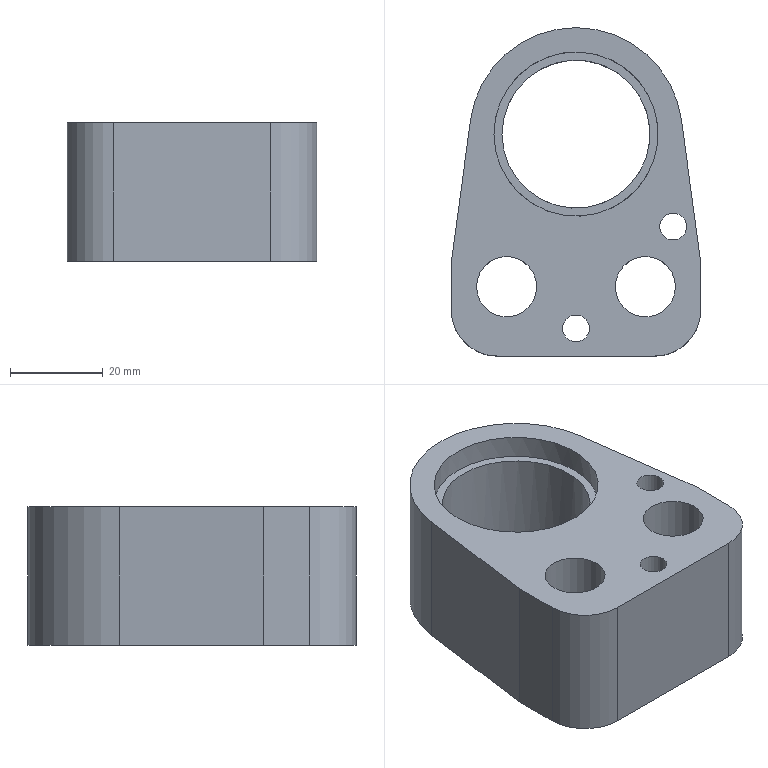Part | NX | features solid 2 | 1 solid | 25 faces | box 54 x 71 x 30 mm | volume 58450 mm3 | cylinder 13 | plane 12 | commonest cylinder face diameters 5.8 x2 8 x2 13 x2 19 x2 20 x2 32 x1
STEP:
#1=CARTESIAN_POINT('',(83.431,151.38,95.));
#2=VERTEX_POINT('',#1);
#3=CARTESIAN_POINT('',(79.223,182.47,95.));
#4=VERTEX_POINT('',#3);
#5=CARTESIAN_POINT('',(80.748,171.199,95.));
#6=DIRECTION('',(-0.1341,0.991,0.));
#7=VECTOR('',#6,1000.);
#8=LINE('',#5,#7);
#9=EDGE_CURVE('',#2,#4,#8,.T.);
#10=ORIENTED_EDGE('',*,*,#9,.T.);
#11=CARTESIAN_POINT('',(33.64,182.47,95.));
#12=VERTEX_POINT('',#11);
#13=CARTESIAN_POINT('',(56.431,179.38,95.));
#14=DIRECTION('',(0.,0.,-1.));
#15=DIRECTION('',(-1.,0.,0.));
#16=AXIS2_PLACEMENT_3D('',#13,#14,#15);
#17=CIRCLE('',#16,23.);
#18=EDGE_CURVE('',#12,#4,#17,.T.);
#19=ORIENTED_EDGE('',*,*,#18,.F.);
#20=CARTESIAN_POINT('',(29.431,151.38,95.));
#21=VERTEX_POINT('',#20);
#22=CARTESIAN_POINT('',(32.114,171.199,95.));
#23=DIRECTION('',(-0.1341,-0.991,0.));
#24=VECTOR('',#23,1000.);
#25=LINE('',#22,#24);
#26=EDGE_CURVE('',#12,#21,#25,.T.);
#27=ORIENTED_EDGE('',*,*,#26,.T.);
#28=CARTESIAN_POINT('',(29.431,141.38,95.));
#29=VERTEX_POINT('',#28);
#30=CARTESIAN_POINT('',(29.431,166.925,95.));
#31=DIRECTION('',(0.,1.,0.));
#32=VECTOR('',#31,1000.);
#33=LINE('',#30,#32);
#34=EDGE_CURVE('',#29,#21,#33,.T.);
#35=ORIENTED_EDGE('',*,*,#34,.F.);
#36=CARTESIAN_POINT('',(39.431,131.38,95.));
#37=VERTEX_POINT('',#36);
#38=CARTESIAN_POINT('',(39.431,141.38,95.));
#39=DIRECTION('',(0.,0.,1.));
#40=DIRECTION('',(1.,0.,0.));
#41=AXIS2_PLACEMENT_3D('',#38,#39,#40);
#42=CIRCLE('',#41,10.);
#43=EDGE_CURVE('',#29,#37,#42,.T.);
#44=ORIENTED_EDGE('',*,*,#43,.T.);
#45=CARTESIAN_POINT('',(73.431,131.38,95.));
#46=VERTEX_POINT('',#45);
#47=CARTESIAN_POINT('',(56.431,131.38,95.));
#48=DIRECTION('',(-1.,0.,0.));
#49=VECTOR('',#48,1000.);
#50=LINE('',#47,#49);
#51=EDGE_CURVE('',#46,#37,#50,.T.);
#52=ORIENTED_EDGE('',*,*,#51,.F.);
#53=CARTESIAN_POINT('',(83.431,141.38,95.));
#54=VERTEX_POINT('',#53);
#55=CARTESIAN_POINT('',(73.431,141.38,95.));
#56=DIRECTION('',(0.,0.,1.));
#57=DIRECTION('',(1.,0.,0.));
#58=AXIS2_PLACEMENT_3D('',#55,#56,#57);
#59=CIRCLE('',#58,10.);
#60=EDGE_CURVE('',#46,#54,#59,.T.);
#61=ORIENTED_EDGE('',*,*,#60,.T.);
#62=CARTESIAN_POINT('',(83.431,166.925,95.));
#63=DIRECTION('',(0.,-1.,0.));
#64=VECTOR('',#63,1000.);
#65=LINE('',#62,#64);
#66=EDGE_CURVE('',#2,#54,#65,.T.);
#67=ORIENTED_EDGE('',*,*,#66,.F.);
#68=EDGE_LOOP('',(#10,#19,#27,#35,#44,#52,#61,#67));
#69=FACE_BOUND('',#68,.T.);
#70=CARTESIAN_POINT('',(53.531,137.38,95.));
#71=VERTEX_POINT('',#70);
#72=CARTESIAN_POINT('',(56.431,137.38,95.));
#73=DIRECTION('',(0.,0.,-1.));
#74=DIRECTION('',(-1.,0.,0.));
#75=AXIS2_PLACEMENT_3D('',#72,#73,#74);
#76=CIRCLE('',#75,2.9);
#77=EDGE_CURVE('',#71,#71,#76,.T.);
#78=ORIENTED_EDGE('',*,*,#77,.T.);
#79=EDGE_LOOP('',(#78));
#80=FACE_BOUND('',#79,.T.);
#81=CARTESIAN_POINT('',(74.531,159.38,95.));
#82=VERTEX_POINT('',#81);
#83=CARTESIAN_POINT('',(77.431,159.38,95.));
#84=DIRECTION('',(0.,0.,-1.));
#85=DIRECTION('',(-1.,0.,0.));
#86=AXIS2_PLACEMENT_3D('',#83,#84,#85);
#87=CIRCLE('',#86,2.9);
#88=EDGE_CURVE('',#82,#82,#87,.T.);
#89=ORIENTED_EDGE('',*,*,#88,.T.);
#90=EDGE_LOOP('',(#89));
#91=FACE_BOUND('',#90,.T.);
#92=CARTESIAN_POINT('',(64.931,146.38,95.));
#93=VERTEX_POINT('',#92);
#94=CARTESIAN_POINT('',(71.431,146.38,95.));
#95=DIRECTION('',(0.,0.,-1.));
#96=DIRECTION('',(-1.,0.,0.));
#97=AXIS2_PLACEMENT_3D('',#94,#95,#96);
#98=CIRCLE('',#97,6.5);
#99=EDGE_CURVE('',#93,#93,#98,.T.);
#100=ORIENTED_EDGE('',*,*,#99,.T.);
#101=EDGE_LOOP('',(#100));
#102=FACE_BOUND('',#101,.T.);
#103=CARTESIAN_POINT('',(34.931,146.38,95.));
#104=VERTEX_POINT('',#103);
#105=CARTESIAN_POINT('',(41.431,146.38,95.));
#106=DIRECTION('',(0.,0.,-1.));
#107=DIRECTION('',(-1.,0.,0.));
#108=AXIS2_PLACEMENT_3D('',#105,#106,#107);
#109=CIRCLE('',#108,6.5);
#110=EDGE_CURVE('',#104,#104,#109,.T.);
#111=ORIENTED_EDGE('',*,*,#110,.T.);
#112=EDGE_LOOP('',(#111));
#113=FACE_BOUND('',#112,.T.);
#114=CARTESIAN_POINT('',(38.681,179.38,95.));
#115=VERTEX_POINT('',#114);
#116=CARTESIAN_POINT('',(56.431,179.38,95.));
#117=DIRECTION('',(0.,0.,-1.));
#118=DIRECTION('',(-1.,0.,0.));
#119=AXIS2_PLACEMENT_3D('',#116,#117,#118);
#120=CIRCLE('',#119,17.75);
#121=EDGE_CURVE('',#115,#115,#120,.T.);
#122=ORIENTED_EDGE('',*,*,#121,.T.);
#123=EDGE_LOOP('',(#122));
#124=FACE_BOUND('',#123,.T.);
#125=CARTESIAN_POINT('',(56.431,166.925,95.));
#126=DIRECTION('',(0.,0.,1.));
#127=DIRECTION('',(1.,0.,0.));
#128=AXIS2_PLACEMENT_3D('',#125,#126,#127);
#129=PLANE('',#128);
#130=ADVANCED_FACE('',(#69,#80,#91,#102,#113,#124),#129,.T.);
#131=CARTESIAN_POINT('',(29.431,151.38,65.));
#132=VERTEX_POINT('',#131);
#133=CARTESIAN_POINT('',(29.431,151.38,65.));
#134=DIRECTION('',(0.,0.,1.));
#135=VECTOR('',#134,1000.);
#136=LINE('',#133,#135);
#137=EDGE_CURVE('',#132,#21,#136,.T.);
#138=ORIENTED_EDGE('',*,*,#137,.F.);
#139=CARTESIAN_POINT('',(29.431,141.38,65.));
#140=VERTEX_POINT('',#139);
#141=CARTESIAN_POINT('',(29.431,166.925,65.));
#142=DIRECTION('',(0.,-1.,0.));
#143=VECTOR('',#142,1000.);
#144=LINE('',#141,#143);
#145=EDGE_CURVE('',#132,#140,#144,.T.);
#146=ORIENTED_EDGE('',*,*,#145,.T.);
#147=CARTESIAN_POINT('',(29.431,141.38,65.));
#148=DIRECTION('',(0.,0.,1.));
#149=VECTOR('',#148,1000.);
#150=LINE('',#147,#149);
#151=EDGE_CURVE('',#140,#29,#150,.T.);
#152=ORIENTED_EDGE('',*,*,#151,.T.);
#153=ORIENTED_EDGE('',*,*,#34,.T.);
#154=EDGE_LOOP('',(#138,#146,#152,#153));
#155=FACE_BOUND('',#154,.T.);
#156=CARTESIAN_POINT('',(29.431,166.925,65.));
#157=DIRECTION('',(-1.,0.,0.));
#158=DIRECTION('',(0.,0.,1.));
#159=AXIS2_PLACEMENT_3D('',#156,#157,#158);
#160=PLANE('',#159);
#161=ADVANCED_FACE('',(#155),#160,.T.);
#162=CARTESIAN_POINT('',(79.223,182.47,65.));
#163=VERTEX_POINT('',#162);
#164=CARTESIAN_POINT('',(83.431,151.38,65.));
#165=VERTEX_POINT('',#164);
#166=CARTESIAN_POINT('',(80.748,171.199,65.));
#167=DIRECTION('',(0.1341,-0.991,0.));
#168=VECTOR('',#167,1000.);
#169=LINE('',#166,#168);
#170=EDGE_CURVE('',#163,#165,#169,.T.);
#171=ORIENTED_EDGE('',*,*,#170,.T.);
#172=CARTESIAN_POINT('',(83.431,141.38,65.));
#173=VERTEX_POINT('',#172);
#174=CARTESIAN_POINT('',(83.431,166.925,65.));
#175=DIRECTION('',(0.,1.,0.));
#176=VECTOR('',#175,1000.);
#177=LINE('',#174,#176);
#178=EDGE_CURVE('',#173,#165,#177,.T.);
#179=ORIENTED_EDGE('',*,*,#178,.F.);
#180=CARTESIAN_POINT('',(73.431,131.38,65.));
#181=VERTEX_POINT('',#180);
#182=CARTESIAN_POINT('',(73.431,141.38,65.));
#183=DIRECTION('',(0.,0.,-1.));
#184=DIRECTION('',(-1.,0.,0.));
#185=AXIS2_PLACEMENT_3D('',#182,#183,#184);
#186=CIRCLE('',#185,10.);
#187=EDGE_CURVE('',#173,#181,#186,.T.);
#188=ORIENTED_EDGE('',*,*,#187,.T.);
#189=CARTESIAN_POINT('',(39.431,131.38,65.));
#190=VERTEX_POINT('',#189);
#191=CARTESIAN_POINT('',(56.431,131.38,65.));
#192=DIRECTION('',(1.,0.,0.));
#193=VECTOR('',#192,1000.);
#194=LINE('',#191,#193);
#195=EDGE_CURVE('',#190,#181,#194,.T.);
#196=ORIENTED_EDGE('',*,*,#195,.F.);
#197=CARTESIAN_POINT('',(39.431,141.38,65.));
#198=DIRECTION('',(0.,0.,-1.));
#199=DIRECTION('',(-1.,0.,0.));
#200=AXIS2_PLACEMENT_3D('',#197,#198,#199);
#201=CIRCLE('',#200,10.);
#202=EDGE_CURVE('',#190,#140,#201,.T.);
#203=ORIENTED_EDGE('',*,*,#202,.T.);
#204=ORIENTED_EDGE('',*,*,#145,.F.);
#205=CARTESIAN_POINT('',(33.64,182.47,65.));
#206=VERTEX_POINT('',#205);
#207=CARTESIAN_POINT('',(32.114,171.199,65.));
#208=DIRECTION('',(0.1341,0.991,0.));
#209=VECTOR('',#208,1000.);
#210=LINE('',#207,#209);
#211=EDGE_CURVE('',#132,#206,#210,.T.);
#212=ORIENTED_EDGE('',*,*,#211,.T.);
#213=CARTESIAN_POINT('',(56.431,179.38,65.));
#214=DIRECTION('',(0.,0.,1.));
#215=DIRECTION('',(1.,0.,0.));
#216=AXIS2_PLACEMENT_3D('',#213,#214,#215);
#217=CIRCLE('',#216,23.);
#218=EDGE_CURVE('',#163,#206,#217,.T.);
#219=ORIENTED_EDGE('',*,*,#218,.F.);
#220=EDGE_LOOP('',(#171,#179,#188,#196,#203,#204,#212,#219));
#221=FACE_BOUND('',#220,.T.);
#222=CARTESIAN_POINT('',(60.431,137.38,65.));
#223=VERTEX_POINT('',#222);
#224=CARTESIAN_POINT('',(56.431,137.38,65.));
#225=DIRECTION('',(0.,0.,1.));
#226=DIRECTION('',(1.,0.,0.));
#227=AXIS2_PLACEMENT_3D('',#224,#225,#226);
#228=CIRCLE('',#227,4.);
#229=EDGE_CURVE('',#223,#223,#228,.T.);
#230=ORIENTED_EDGE('',*,*,#229,.T.);
#231=EDGE_LOOP('',(#230));
#232=FACE_BOUND('',#231,.T.);
#233=CARTESIAN_POINT('',(81.431,159.38,65.));
#234=VERTEX_POINT('',#233);
#235=CARTESIAN_POINT('',(77.431,159.38,65.));
#236=DIRECTION('',(0.,0.,1.));
#237=DIRECTION('',(1.,0.,0.));
#238=AXIS2_PLACEMENT_3D('',#235,#236,#237);
#239=CIRCLE('',#238,4.);
#240=EDGE_CURVE('',#234,#234,#239,.T.);
#241=ORIENTED_EDGE('',*,*,#240,.T.);
#242=EDGE_LOOP('',(#241));
#243=FACE_BOUND('',#242,.T.);
#244=CARTESIAN_POINT('',(80.931,146.38,65.));
#245=VERTEX_POINT('',#244);
#246=CARTESIAN_POINT('',(71.431,146.38,65.));
#247=DIRECTION('',(0.,0.,1.));
#248=DIRECTION('',(1.,0.,0.));
#249=AXIS2_PLACEMENT_3D('',#246,#247,#248);
#250=CIRCLE('',#249,9.5);
#251=EDGE_CURVE('',#245,#245,#250,.T.);
#252=ORIENTED_EDGE('',*,*,#251,.T.);
#253=EDGE_LOOP('',(#252));
#254=FACE_BOUND('',#253,.T.);
#255=CARTESIAN_POINT('',(50.931,146.38,65.));
#256=VERTEX_POINT('',#255);
#257=CARTESIAN_POINT('',(41.431,146.38,65.));
#258=DIRECTION('',(0.,0.,1.));
#259=DIRECTION('',(1.,0.,0.));
#260=AXIS2_PLACEMENT_3D('',#257,#258,#259);
#261=CIRCLE('',#260,9.5);
#262=EDGE_CURVE('',#256,#256,#261,.T.);
#263=ORIENTED_EDGE('',*,*,#262,.T.);
#264=EDGE_LOOP('',(#263));
#265=FACE_BOUND('',#264,.T.);
#266=CARTESIAN_POINT('',(72.431,179.38,65.));
#267=VERTEX_POINT('',#266);
#268=CARTESIAN_POINT('',(56.431,179.38,65.));
#269=DIRECTION('',(0.,0.,1.));
#270=DIRECTION('',(1.,0.,0.));
#271=AXIS2_PLACEMENT_3D('',#268,#269,#270);
#272=CIRCLE('',#271,16.);
#273=EDGE_CURVE('',#267,#267,#272,.T.);
#274=ORIENTED_EDGE('',*,*,#273,.T.);
#275=EDGE_LOOP('',(#274));
#276=FACE_BOUND('',#275,.T.);
#277=CARTESIAN_POINT('',(56.431,166.925,65.));
#278=DIRECTION('',(0.,0.,-1.));
#279=DIRECTION('',(-1.,0.,0.));
#280=AXIS2_PLACEMENT_3D('',#277,#278,#279);
#281=PLANE('',#280);
#282=ADVANCED_FACE('',(#221,#232,#243,#254,#265,#276),#281,.T.);
#283=CARTESIAN_POINT('',(83.431,151.38,65.));
#284=DIRECTION('',(0.,0.,1.));
#285=VECTOR('',#284,1000.);
#286=LINE('',#283,#285);
#287=EDGE_CURVE('',#165,#2,#286,.T.);
#288=ORIENTED_EDGE('',*,*,#287,.T.);
#289=ORIENTED_EDGE('',*,*,#66,.T.);
#290=CARTESIAN_POINT('',(83.431,141.38,65.));
#291=DIRECTION('',(0.,0.,1.));
#292=VECTOR('',#291,1000.);
#293=LINE('',#290,#292);
#294=EDGE_CURVE('',#54,#173,#293,.F.);
#295=ORIENTED_EDGE('',*,*,#294,.T.);
#296=ORIENTED_EDGE('',*,*,#178,.T.);
#297=EDGE_LOOP('',(#288,#289,#295,#296));
#298=FACE_BOUND('',#297,.T.);
#299=CARTESIAN_POINT('',(83.431,166.925,65.));
#300=DIRECTION('',(1.,0.,0.));
#301=DIRECTION('',(0.,0.,-1.));
#302=AXIS2_PLACEMENT_3D('',#299,#300,#301);
#303=PLANE('',#302);
#304=ADVANCED_FACE('',(#298),#303,.T.);
#305=ORIENTED_EDGE('',*,*,#18,.T.);
#306=CARTESIAN_POINT('',(79.223,182.47,95.));
#307=DIRECTION('',(0.,0.,-1.));
#308=VECTOR('',#307,1000.);
#309=LINE('',#306,#308);
#310=EDGE_CURVE('',#4,#163,#309,.T.);
#311=ORIENTED_EDGE('',*,*,#310,.T.);
#312=ORIENTED_EDGE('',*,*,#218,.T.);
#313=CARTESIAN_POINT('',(33.64,182.47,95.));
#314=DIRECTION('',(0.,0.,-1.));
#315=VECTOR('',#314,1000.);
#316=LINE('',#313,#315);
#317=EDGE_CURVE('',#206,#12,#316,.F.);
#318=ORIENTED_EDGE('',*,*,#317,.T.);
#319=EDGE_LOOP('',(#305,#311,#312,#318));
#320=FACE_BOUND('',#319,.T.);
#321=CARTESIAN_POINT('',(56.431,179.38,95.));
#322=DIRECTION('',(0.,0.,-1.));
#323=DIRECTION('',(-1.,0.,0.));
#324=AXIS2_PLACEMENT_3D('',#321,#322,#323);
#325=CYLINDRICAL_SURFACE('',#324,23.);
#326=ADVANCED_FACE('',(#320),#325,.T.);
#327=ORIENTED_EDGE('',*,*,#195,.T.);
#328=CARTESIAN_POINT('',(73.431,131.38,65.));
#329=DIRECTION('',(0.,0.,1.));
#330=VECTOR('',#329,1000.);
#331=LINE('',#328,#330);
#332=EDGE_CURVE('',#181,#46,#331,.T.);
#333=ORIENTED_EDGE('',*,*,#332,.T.);
#334=ORIENTED_EDGE('',*,*,#51,.T.);
#335=CARTESIAN_POINT('',(39.431,131.38,65.));
#336=DIRECTION('',(0.,0.,1.));
#337=VECTOR('',#336,1000.);
#338=LINE('',#335,#337);
#339=EDGE_CURVE('',#37,#190,#338,.F.);
#340=ORIENTED_EDGE('',*,*,#339,.T.);
#341=EDGE_LOOP('',(#327,#333,#334,#340));
#342=FACE_BOUND('',#341,.T.);
#343=CARTESIAN_POINT('',(56.431,131.38,65.));
#344=DIRECTION('',(0.,-1.,0.));
#345=DIRECTION('',(0.,0.,-1.));
#346=AXIS2_PLACEMENT_3D('',#343,#344,#345);
#347=PLANE('',#346);
#348=ADVANCED_FACE('',(#342),#347,.T.);
#349=CARTESIAN_POINT('',(40.431,179.38,90.));
#350=VERTEX_POINT('',#349);
#351=CARTESIAN_POINT('',(56.431,179.38,90.));
#352=DIRECTION('',(0.,0.,-1.));
#353=DIRECTION('',(-1.,0.,0.));
#354=AXIS2_PLACEMENT_3D('',#351,#352,#353);
#355=CIRCLE('',#354,16.);
#356=EDGE_CURVE('',#350,#350,#355,.T.);
#357=ORIENTED_EDGE('',*,*,#356,.T.);
#358=EDGE_LOOP('',(#357));
#359=FACE_BOUND('',#358,.T.);
#360=CARTESIAN_POINT('',(74.181,179.38,90.));
#361=VERTEX_POINT('',#360);
#362=CARTESIAN_POINT('',(56.431,179.38,90.));
#363=DIRECTION('',(0.,0.,1.));
#364=DIRECTION('',(1.,0.,0.));
#365=AXIS2_PLACEMENT_3D('',#362,#363,#364);
#366=CIRCLE('',#365,17.75);
#367=EDGE_CURVE('',#361,#361,#366,.T.);
#368=ORIENTED_EDGE('',*,*,#367,.T.);
#369=EDGE_LOOP('',(#368));
#370=FACE_BOUND('',#369,.T.);
#371=CARTESIAN_POINT('',(56.431,179.38,90.));
#372=DIRECTION('',(0.,0.,-1.));
#373=DIRECTION('',(-1.,0.,0.));
#374=AXIS2_PLACEMENT_3D('',#371,#372,#373);
#375=PLANE('',#374);
#376=ADVANCED_FACE('',(#359,#370),#375,.F.);
#377=ORIENTED_EDGE('',*,*,#367,.F.);
#378=EDGE_LOOP('',(#377));
#379=FACE_BOUND('',#378,.T.);
#380=ORIENTED_EDGE('',*,*,#121,.F.);
#381=EDGE_LOOP('',(#380));
#382=FACE_BOUND('',#381,.T.);
#383=CARTESIAN_POINT('',(56.431,179.38,95.));
#384=DIRECTION('',(0.,0.,-1.));
#385=DIRECTION('',(-1.,0.,0.));
#386=AXIS2_PLACEMENT_3D('',#383,#384,#385);
#387=CYLINDRICAL_SURFACE('',#386,17.75);
#388=ADVANCED_FACE('',(#379,#382),#387,.F.);
#389=ORIENTED_EDGE('',*,*,#273,.F.);
#390=EDGE_LOOP('',(#389));
#391=FACE_BOUND('',#390,.T.);
#392=ORIENTED_EDGE('',*,*,#356,.F.);
#393=EDGE_LOOP('',(#392));
#394=FACE_BOUND('',#393,.T.);
#395=CARTESIAN_POINT('',(56.431,179.38,90.));
#396=DIRECTION('',(0.,0.,-1.));
#397=DIRECTION('',(-1.,0.,0.));
#398=AXIS2_PLACEMENT_3D('',#395,#396,#397);
#399=CYLINDRICAL_SURFACE('',#398,16.);
#400=ADVANCED_FACE('',(#391,#394),#399,.F.);
#401=CARTESIAN_POINT('',(47.931,146.38,79.));
#402=VERTEX_POINT('',#401);
#403=CARTESIAN_POINT('',(41.431,146.38,79.));
#404=DIRECTION('',(0.,0.,1.));
#405=DIRECTION('',(1.,0.,0.));
#406=AXIS2_PLACEMENT_3D('',#403,#404,#405);
#407=CIRCLE('',#406,6.5);
#408=EDGE_CURVE('',#402,#402,#407,.F.);
#409=ORIENTED_EDGE('',*,*,#408,.T.);
#410=EDGE_LOOP('',(#409));
#411=FACE_BOUND('',#410,.T.);
#412=ORIENTED_EDGE('',*,*,#110,.F.);
#413=EDGE_LOOP('',(#412));
#414=FACE_BOUND('',#413,.T.);
#415=CARTESIAN_POINT('',(41.431,146.38,95.));
#416=DIRECTION('',(0.,0.,-1.));
#417=DIRECTION('',(-1.,0.,0.));
#418=AXIS2_PLACEMENT_3D('',#415,#416,#417);
#419=CYLINDRICAL_SURFACE('',#418,6.5);
#420=ADVANCED_FACE('',(#411,#414),#419,.F.);
#421=CARTESIAN_POINT('',(31.931,146.38,79.));
#422=VERTEX_POINT('',#421);
#423=CARTESIAN_POINT('',(41.431,146.38,79.));
#424=DIRECTION('',(0.,0.,-1.));
#425=DIRECTION('',(-1.,0.,0.));
#426=AXIS2_PLACEMENT_3D('',#423,#424,#425);
#427=CIRCLE('',#426,9.5);
#428=EDGE_CURVE('',#422,#422,#427,.T.);
#429=ORIENTED_EDGE('',*,*,#428,.T.);
#430=EDGE_LOOP('',(#429));
#431=FACE_BOUND('',#430,.T.);
#432=ORIENTED_EDGE('',*,*,#408,.F.);
#433=EDGE_LOOP('',(#432));
#434=FACE_BOUND('',#433,.T.);
#435=CARTESIAN_POINT('',(41.431,146.38,79.));
#436=DIRECTION('',(0.,0.,1.));
#437=DIRECTION('',(1.,0.,0.));
#438=AXIS2_PLACEMENT_3D('',#435,#436,#437);
#439=PLANE('',#438);
#440=ADVANCED_FACE('',(#431,#434),#439,.F.);
#441=ORIENTED_EDGE('',*,*,#262,.F.);
#442=EDGE_LOOP('',(#441));
#443=FACE_BOUND('',#442,.T.);
#444=ORIENTED_EDGE('',*,*,#428,.F.);
#445=EDGE_LOOP('',(#444));
#446=FACE_BOUND('',#445,.T.);
#447=CARTESIAN_POINT('',(41.431,146.38,79.));
#448=DIRECTION('',(0.,0.,-1.));
#449=DIRECTION('',(-1.,0.,0.));
#450=AXIS2_PLACEMENT_3D('',#447,#448,#449);
#451=CYLINDRICAL_SURFACE('',#450,9.5);
#452=ADVANCED_FACE('',(#443,#446),#451,.F.);
#453=CARTESIAN_POINT('',(77.931,146.38,79.));
#454=VERTEX_POINT('',#453);
#455=CARTESIAN_POINT('',(71.431,146.38,79.));
#456=DIRECTION('',(0.,0.,1.));
#457=DIRECTION('',(1.,0.,0.));
#458=AXIS2_PLACEMENT_3D('',#455,#456,#457);
#459=CIRCLE('',#458,6.5);
#460=EDGE_CURVE('',#454,#454,#459,.F.);
#461=ORIENTED_EDGE('',*,*,#460,.T.);
#462=EDGE_LOOP('',(#461));
#463=FACE_BOUND('',#462,.T.);
#464=ORIENTED_EDGE('',*,*,#99,.F.);
#465=EDGE_LOOP('',(#464));
#466=FACE_BOUND('',#465,.T.);
#467=CARTESIAN_POINT('',(71.431,146.38,95.));
#468=DIRECTION('',(0.,0.,-1.));
#469=DIRECTION('',(-1.,0.,0.));
#470=AXIS2_PLACEMENT_3D('',#467,#468,#469);
#471=CYLINDRICAL_SURFACE('',#470,6.5);
#472=ADVANCED_FACE('',(#463,#466),#471,.F.);
#473=CARTESIAN_POINT('',(61.931,146.38,79.));
#474=VERTEX_POINT('',#473);
#475=CARTESIAN_POINT('',(71.431,146.38,79.));
#476=DIRECTION('',(0.,0.,-1.));
#477=DIRECTION('',(-1.,0.,0.));
#478=AXIS2_PLACEMENT_3D('',#475,#476,#477);
#479=CIRCLE('',#478,9.5);
#480=EDGE_CURVE('',#474,#474,#479,.T.);
#481=ORIENTED_EDGE('',*,*,#480,.T.);
#482=EDGE_LOOP('',(#481));
#483=FACE_BOUND('',#482,.T.);
#484=ORIENTED_EDGE('',*,*,#460,.F.);
#485=EDGE_LOOP('',(#484));
#486=FACE_BOUND('',#485,.T.);
#487=CARTESIAN_POINT('',(71.431,146.38,79.));
#488=DIRECTION('',(0.,0.,1.));
#489=DIRECTION('',(1.,0.,0.));
#490=AXIS2_PLACEMENT_3D('',#487,#488,#489);
#491=PLANE('',#490);
#492=ADVANCED_FACE('',(#483,#486),#491,.F.);
#493=ORIENTED_EDGE('',*,*,#251,.F.);
#494=EDGE_LOOP('',(#493));
#495=FACE_BOUND('',#494,.T.);
#496=ORIENTED_EDGE('',*,*,#480,.F.);
#497=EDGE_LOOP('',(#496));
#498=FACE_BOUND('',#497,.T.);
#499=CARTESIAN_POINT('',(71.431,146.38,79.));
#500=DIRECTION('',(0.,0.,-1.));
#501=DIRECTION('',(-1.,0.,0.));
#502=AXIS2_PLACEMENT_3D('',#499,#500,#501);
#503=CYLINDRICAL_SURFACE('',#502,9.5);
#504=ADVANCED_FACE('',(#495,#498),#503,.F.);
#505=CARTESIAN_POINT('',(80.331,159.38,85.));
#506=VERTEX_POINT('',#505);
#507=CARTESIAN_POINT('',(77.431,159.38,85.));
#508=DIRECTION('',(0.,0.,1.));
#509=DIRECTION('',(1.,0.,0.));
#510=AXIS2_PLACEMENT_3D('',#507,#508,#509);
#511=CIRCLE('',#510,2.9);
#512=EDGE_CURVE('',#506,#506,#511,.F.);
#513=ORIENTED_EDGE('',*,*,#512,.T.);
#514=EDGE_LOOP('',(#513));
#515=FACE_BOUND('',#514,.T.);
#516=ORIENTED_EDGE('',*,*,#88,.F.);
#517=EDGE_LOOP('',(#516));
#518=FACE_BOUND('',#517,.T.);
#519=CARTESIAN_POINT('',(77.431,159.38,95.));
#520=DIRECTION('',(0.,0.,-1.));
#521=DIRECTION('',(-1.,0.,0.));
#522=AXIS2_PLACEMENT_3D('',#519,#520,#521);
#523=CYLINDRICAL_SURFACE('',#522,2.9);
#524=ADVANCED_FACE('',(#515,#518),#523,.F.);
#525=CARTESIAN_POINT('',(73.431,159.38,85.));
#526=VERTEX_POINT('',#525);
#527=CARTESIAN_POINT('',(77.431,159.38,85.));
#528=DIRECTION('',(0.,0.,-1.));
#529=DIRECTION('',(-1.,0.,0.));
#530=AXIS2_PLACEMENT_3D('',#527,#528,#529);
#531=CIRCLE('',#530,4.);
#532=EDGE_CURVE('',#526,#526,#531,.T.);
#533=ORIENTED_EDGE('',*,*,#532,.T.);
#534=EDGE_LOOP('',(#533));
#535=FACE_BOUND('',#534,.T.);
#536=ORIENTED_EDGE('',*,*,#512,.F.);
#537=EDGE_LOOP('',(#536));
#538=FACE_BOUND('',#537,.T.);
#539=CARTESIAN_POINT('',(77.431,159.38,85.));
#540=DIRECTION('',(0.,0.,1.));
#541=DIRECTION('',(1.,0.,0.));
#542=AXIS2_PLACEMENT_3D('',#539,#540,#541);
#543=PLANE('',#542);
#544=ADVANCED_FACE('',(#535,#538),#543,.F.);
#545=ORIENTED_EDGE('',*,*,#240,.F.);
#546=EDGE_LOOP('',(#545));
#547=FACE_BOUND('',#546,.T.);
#548=ORIENTED_EDGE('',*,*,#532,.F.);
#549=EDGE_LOOP('',(#548));
#550=FACE_BOUND('',#549,.T.);
#551=CARTESIAN_POINT('',(77.431,159.38,85.));
#552=DIRECTION('',(0.,0.,-1.));
#553=DIRECTION('',(-1.,0.,0.));
#554=AXIS2_PLACEMENT_3D('',#551,#552,#553);
#555=CYLINDRICAL_SURFACE('',#554,4.);
#556=ADVANCED_FACE('',(#547,#550),#555,.F.);
#557=CARTESIAN_POINT('',(59.331,137.38,85.));
#558=VERTEX_POINT('',#557);
#559=CARTESIAN_POINT('',(56.431,137.38,85.));
#560=DIRECTION('',(0.,0.,1.));
#561=DIRECTION('',(1.,0.,0.));
#562=AXIS2_PLACEMENT_3D('',#559,#560,#561);
#563=CIRCLE('',#562,2.9);
#564=EDGE_CURVE('',#558,#558,#563,.F.);
#565=ORIENTED_EDGE('',*,*,#564,.T.);
#566=EDGE_LOOP('',(#565));
#567=FACE_BOUND('',#566,.T.);
#568=ORIENTED_EDGE('',*,*,#77,.F.);
#569=EDGE_LOOP('',(#568));
#570=FACE_BOUND('',#569,.T.);
#571=CARTESIAN_POINT('',(56.431,137.38,95.));
#572=DIRECTION('',(0.,0.,-1.));
#573=DIRECTION('',(-1.,0.,0.));
#574=AXIS2_PLACEMENT_3D('',#571,#572,#573);
#575=CYLINDRICAL_SURFACE('',#574,2.9);
#576=ADVANCED_FACE('',(#567,#570),#575,.F.);
#577=CARTESIAN_POINT('',(52.431,137.38,85.));
#578=VERTEX_POINT('',#577);
#579=CARTESIAN_POINT('',(56.431,137.38,85.));
#580=DIRECTION('',(0.,0.,-1.));
#581=DIRECTION('',(-1.,0.,0.));
#582=AXIS2_PLACEMENT_3D('',#579,#580,#581);
#583=CIRCLE('',#582,4.);
#584=EDGE_CURVE('',#578,#578,#583,.T.);
#585=ORIENTED_EDGE('',*,*,#584,.T.);
#586=EDGE_LOOP('',(#585));
#587=FACE_BOUND('',#586,.T.);
#588=ORIENTED_EDGE('',*,*,#564,.F.);
#589=EDGE_LOOP('',(#588));
#590=FACE_BOUND('',#589,.T.);
#591=CARTESIAN_POINT('',(56.431,137.38,85.));
#592=DIRECTION('',(0.,0.,1.));
#593=DIRECTION('',(1.,0.,0.));
#594=AXIS2_PLACEMENT_3D('',#591,#592,#593);
#595=PLANE('',#594);
#596=ADVANCED_FACE('',(#587,#590),#595,.F.);
#597=ORIENTED_EDGE('',*,*,#229,.F.);
#598=EDGE_LOOP('',(#597));
#599=FACE_BOUND('',#598,.T.);
#600=ORIENTED_EDGE('',*,*,#584,.F.);
#601=EDGE_LOOP('',(#600));
#602=FACE_BOUND('',#601,.T.);
#603=CARTESIAN_POINT('',(56.431,137.38,85.));
#604=DIRECTION('',(0.,0.,-1.));
#605=DIRECTION('',(-1.,0.,0.));
#606=AXIS2_PLACEMENT_3D('',#603,#604,#605);
#607=CYLINDRICAL_SURFACE('',#606,4.);
#608=ADVANCED_FACE('',(#599,#602),#607,.F.);
#609=ORIENTED_EDGE('',*,*,#187,.F.);
#610=ORIENTED_EDGE('',*,*,#294,.F.);
#611=ORIENTED_EDGE('',*,*,#60,.F.);
#612=ORIENTED_EDGE('',*,*,#332,.F.);
#613=EDGE_LOOP('',(#609,#610,#611,#612));
#614=FACE_BOUND('',#613,.T.);
#615=CARTESIAN_POINT('',(73.431,141.38,65.));
#616=DIRECTION('',(0.,0.,1.));
#617=DIRECTION('',(1.,0.,0.));
#618=AXIS2_PLACEMENT_3D('',#615,#616,#617);
#619=CYLINDRICAL_SURFACE('',#618,10.);
#620=ADVANCED_FACE('',(#614),#619,.T.);
#621=ORIENTED_EDGE('',*,*,#202,.F.);
#622=ORIENTED_EDGE('',*,*,#339,.F.);
#623=ORIENTED_EDGE('',*,*,#43,.F.);
#624=ORIENTED_EDGE('',*,*,#151,.F.);
#625=EDGE_LOOP('',(#621,#622,#623,#624));
#626=FACE_BOUND('',#625,.T.);
#627=CARTESIAN_POINT('',(39.431,141.38,65.));
#628=DIRECTION('',(0.,0.,1.));
#629=DIRECTION('',(1.,0.,0.));
#630=AXIS2_PLACEMENT_3D('',#627,#628,#629);
#631=CYLINDRICAL_SURFACE('',#630,10.);
#632=ADVANCED_FACE('',(#626),#631,.T.);
#633=ORIENTED_EDGE('',*,*,#317,.F.);
#634=ORIENTED_EDGE('',*,*,#211,.F.);
#635=ORIENTED_EDGE('',*,*,#137,.T.);
#636=ORIENTED_EDGE('',*,*,#26,.F.);
#637=EDGE_LOOP('',(#633,#634,#635,#636));
#638=FACE_BOUND('',#637,.T.);
#639=CARTESIAN_POINT('',(32.114,171.199,65.));
#640=DIRECTION('',(0.991,-0.1341,0.));
#641=DIRECTION('',(0.,0.,-1.));
#642=AXIS2_PLACEMENT_3D('',#639,#640,#641);
#643=PLANE('',#642);
#644=ADVANCED_FACE('',(#638),#643,.F.);
#645=ORIENTED_EDGE('',*,*,#310,.F.);
#646=ORIENTED_EDGE('',*,*,#9,.F.);
#647=ORIENTED_EDGE('',*,*,#287,.F.);
#648=ORIENTED_EDGE('',*,*,#170,.F.);
#649=EDGE_LOOP('',(#645,#646,#647,#648));
#650=FACE_BOUND('',#649,.T.);
#651=CARTESIAN_POINT('',(80.748,171.199,65.));
#652=DIRECTION('',(-0.991,-0.1341,0.));
#653=DIRECTION('',(0.,0.,1.));
#654=AXIS2_PLACEMENT_3D('',#651,#652,#653);
#655=PLANE('',#654);
#656=ADVANCED_FACE('',(#650),#655,.F.);
#657=CLOSED_SHELL('',(#130,#161,#282,#304,#326,#348,#376,#388,#400,#420,#440,#452,#472,#492,#504,#524,#544,#556,#576,#596,#608,#620,#632,#644,#656));
#658=MANIFOLD_SOLID_BREP('',#657);
#659=(LENGTH_UNIT()NAMED_UNIT(*)SI_UNIT(.MILLI.,.METRE.));
#660=UNCERTAINTY_MEASURE_WITH_UNIT(LENGTH_MEASURE(0.00001),#659,'','');
#661=(NAMED_UNIT(*)PLANE_ANGLE_UNIT()SI_UNIT($,.RADIAN.));
#662=(NAMED_UNIT(*)SI_UNIT($,.STERADIAN.)SOLID_ANGLE_UNIT());
#663=(GEOMETRIC_REPRESENTATION_CONTEXT(3)GLOBAL_UNCERTAINTY_ASSIGNED_CONTEXT((#660))GLOBAL_UNIT_ASSIGNED_CONTEXT((#659,#661,#662))REPRESENTATION_CONTEXT('',''));
#664=ADVANCED_BREP_SHAPE_REPRESENTATION('',(#658),#663);